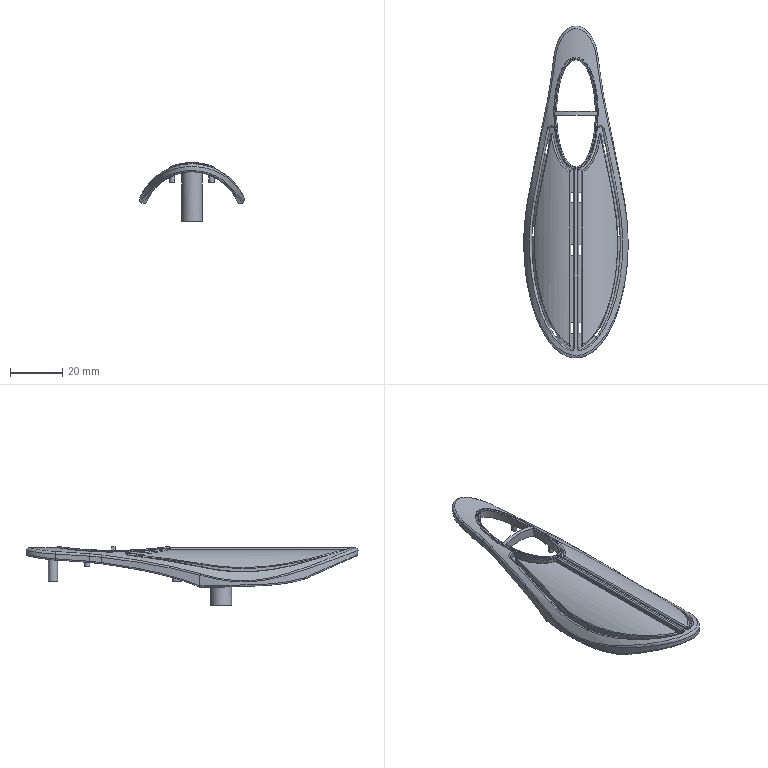Part | STEP file | 1 solid | 213 faces | box 40 x 127.347 x 22.5 mm | volume 10331 mm3 | spline 86 | cylinder 82 | plane 45 | commonest cylinder face diameters 40 x12 39 x10 0.6 x6 1 x6 2 x6 1.6 x4